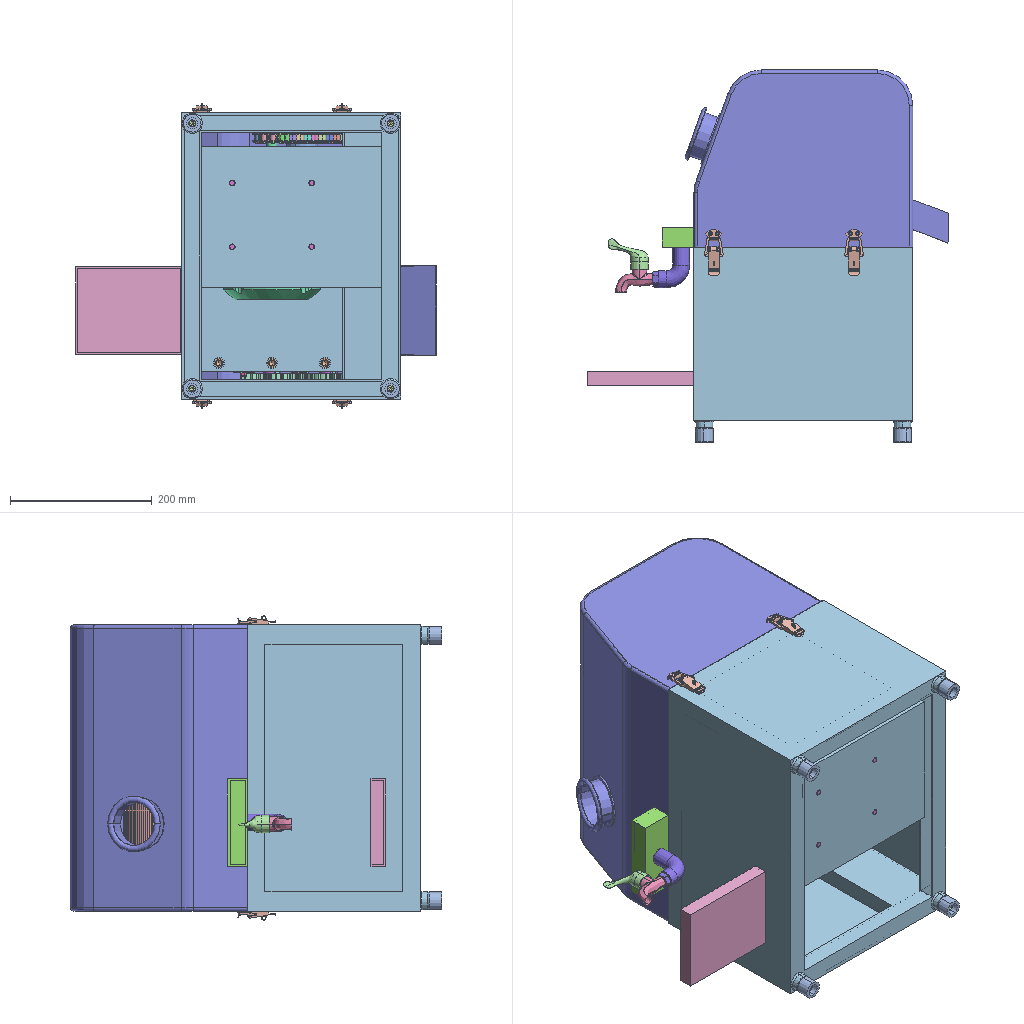Assembly | SolidWorks | 43 different items | 139 placed | box 509 x 525 x 430 mm
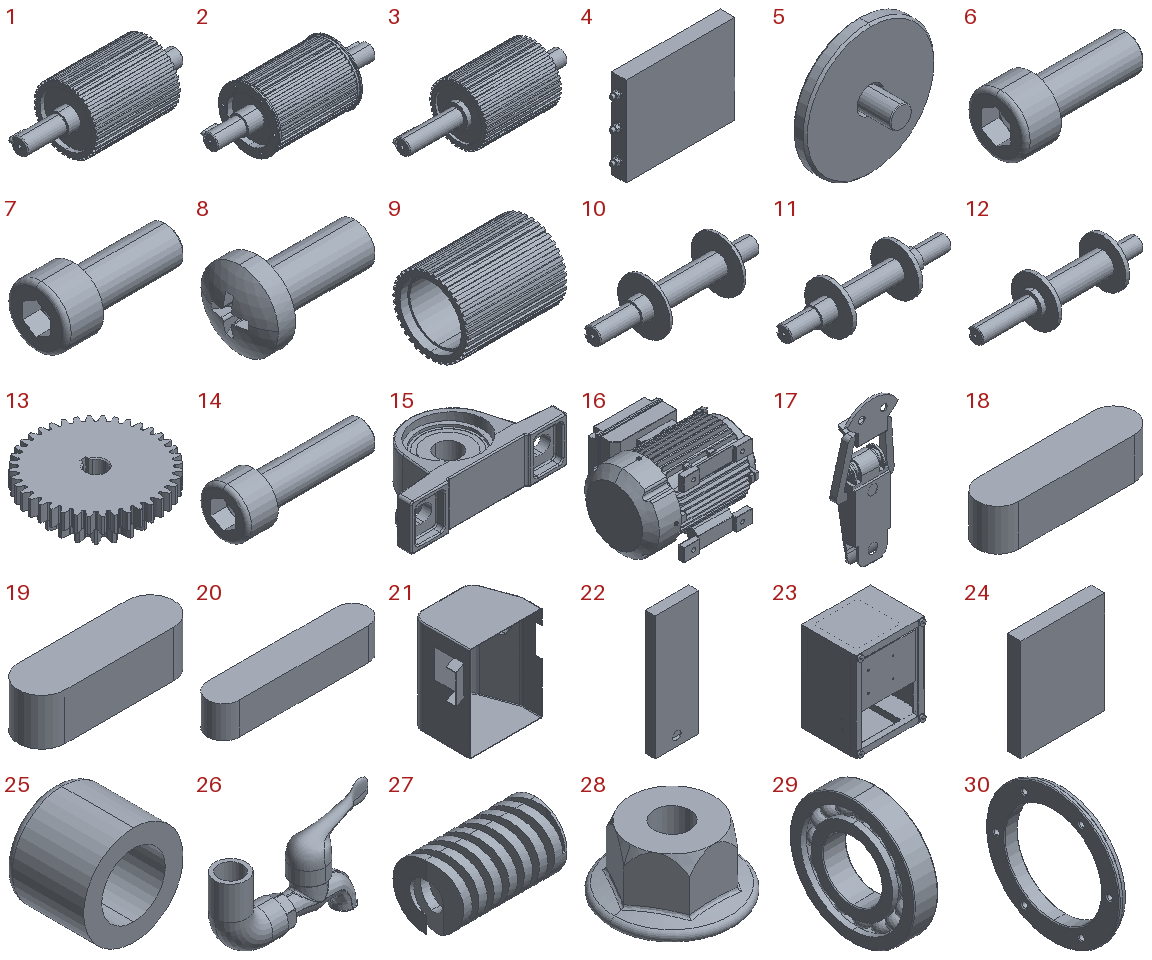Parts list (item | name | quantity | parent item | size | volume | features):
1 | (subassembly) | x1 | - | 188 x 76 x 75.929 mm | 254604 mm3 | -
2 | (subassembly) | x2 | - | 206 x 79 x 79 mm | 296188 mm3 | -
3 | (subassembly) | x1 | - | 211 x 76 x 75.929 mm | 292189 mm3 | -
4 | (subassembly) | x1 | - | 160 x 20 x 123 mm | 58465 mm3 | -
5 | (subassembly) | x10 | - | 30 x 15 x 30 mm | 2467 mm3 | -
6 | - | x4 | - | 22 x 10 x 10 mm | 844.992 mm3 | features BaseBody 1
7 | - | x4 | - | 28 x 13 x 13 mm | 1916 mm3 | features BaseBody 1
8 | - | x3 | in 4 | 15.658 x 9.5 x 9.5 mm | 430.614 mm3 | features BaseBody 1
9 | - | x4 | in 1, 2, 3 | 100 x 76 x 75.929 mm | 159717 mm3 | features BaseBody 1
10 | - | x1 | in 1 | 188 x 62 x 62 mm | 94213 mm3 | features BaseBody 1
11 | - | x2 | in 2 | 206 x 62 x 62 mm | 111425 mm3 | features BaseBody 1
12 | - | x1 | in 3 | 211 x 62 x 62 mm | 131438 mm3 | features BaseBody 1
13 | - | x1 | - | 125.77 x 125.77 x 38 mm | 253321 mm3 | features BaseBody 1
14 | - | x6 | - | 45 x 16 x 16 mm | 4425 mm3 | features BaseBody 1
15 | - | x2 | - | 127 x 73 x 37 mm | 102331 mm3 | features BaseBody 1
16 | - | x1 | - | 240 x 189 x 140.895 mm | 3047126 mm3 | features BaseBody 1
17 | - | x4 | - | 26 x 13 x 64.364 mm | 4721 mm3 | features BaseBody 1
18 | - | x1 | - | 19 x 5 x 5 mm | 448.175 mm3 | features BaseBody 1
19 | - | x7 | in 1, 2 | 20 x 6 x 6 mm | 673.646 mm3 | features BaseBody 1
20 | - | x1 | in 3 | 30 x 6 x 6 mm | 1034 mm3 | features BaseBody 1
21 | - | x1 | - | 371.669 x 250 x 404 mm | 855867 mm3 | features MoveFace 5, BaseBody 1
22 | - | x1 | - | 123 x 28 x 350 mm | 283122 mm3 | features BaseBody 1, DelFace 1, ICE 1, MoveFace 1
23 | - | x1 | - | 309 x 266.4 x 404 mm | 2740160 mm3 | features BaseBody 7, MoveFace 3, Split 2, CombineBodies 1, DelFace 1, ICE 1, MoveCopyBody 1
24 | - | x1 | in 4 | 123 x 20 x 150 mm | 56150 mm3 | features BaseBody 1
25 | - | x4 | - | 25 x 20 x 25 mm | 7114 mm3 | features BaseBody 1
26 | - | x1 | - | - | - | features BaseBody 2, RefSurface 1
27 | - | x4 | - | 35 x 20 x 20 mm | 4844 mm3 | features BaseBody 1
28 | - | x3 | in 4 | 11.8 x 11.8 x 6.2 mm | 341.044 mm3 | features BaseBody 1
29 | - | x8 | - | 8 x 42 x 42 mm | 6601 mm3 | features BaseBody 1
30 | - | x4 | in 2 | 8 x 79 x 79 mm | 11850 mm3 | features BaseBody 1, Chamfer 1, DelFace 1, MoveFace 1
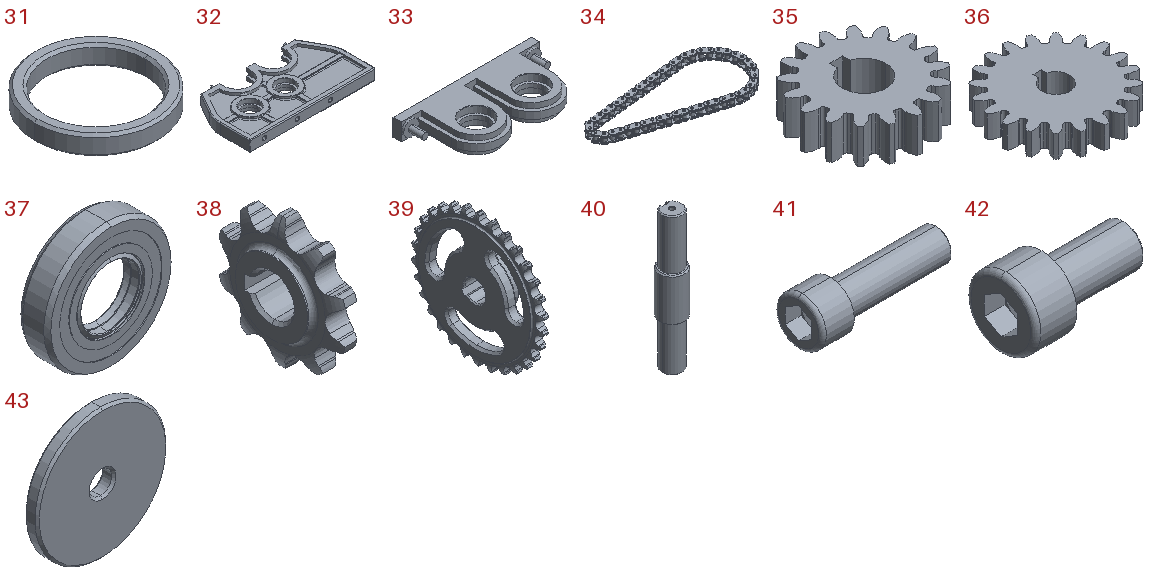31 | - | x9 | - | 25 x 25 x 4 mm | 671.515 mm3 | features BaseBody 1
32 | - | x2 | - | 285 x 151.742 x 25 mm | 571521 mm3 | features ICE 5, MoveFace 2, BaseBody 1, CombineBodies 1, DeleteBody 1, ExtruRefSurface 1, MirrorSolid 1, Split 1
33 | - | x2 | - | 200 x 95.96 x 25 mm | 244043 mm3 | features ICE 2, MoveCopyBody 2, BaseBody 1, CombineBodies 1
34 | - | x1 | - | 290.935 x 132.94 x 17.8 mm | 66914 mm3 | features BaseBody 78
35 | - | x1 | - | 56.683 x 56.908 x 16 mm | 26557 mm3 | features BaseBody 1
36 | - | x5 | - | 87.308 x 87.308 x 16 mm | 73435 mm3 | features BaseBody 1
37 | - | x7 | - | 42 x 10 x 42 mm | 3936 mm3 | features BaseBody 3
38 | - | x1 | - | 11.39 x 43.493 x 45 mm | 8237 mm3 | features BaseBody 1
39 | - | x1 | - | 20.59 x 126.465 x 127 mm | 93015 mm3 | features BaseBody 1
40 | - | x1 | - | 25 x 25 x 138.5 mm | 49958 mm3 | features BaseBody 1
41 | - | x4 | - | 52 x 18 x 18 mm | 6949 mm3 | features BaseBody 1
42 | - | x10 | in 5 | 15 x 8.5 x 8.5 mm | 438.126 mm3 | features BaseBody 1
43 | - | x10 | in 5 | 30 x 3 x 30 mm | 2029 mm3 | features BaseBody 1
Mates (type | each side: item.copy, entity, surface, feature):
Concentric | 32.1 face cylinder Cut-Extrude1 | assembly face
Concentric | assembly face | 36.1 face
Coincident | assembly face | 36.1 face
Parallel | assembly face | 36.1 face
Concentric | assembly face | 43.1 face
Coincident | assembly face | 43.1 face
Concentric | 43.1 face | 42.1 face
Coincident | 43.1 face | 42.1 face
Concentric | 33.1 face cylinder Body-Move/Copy1 | 27.1 face cylinder Input 1
Coincident | 32.2 face plane Input 1 | 27.1 face plane Input 1
Concentric | 33.2 face cylinder Body-Move/Copy1 | 27.2 face cylinder Input 1
Coincident | 32.1 face plane Input 1 | 27.2 face plane Input 1
Width | 22.1 face plane Input 1 | 22.1 face plane Input 1 | 26.1 face cylinder Input 1
Coincident | 22.1 face plane Input 1 | 26.1 face plane Input 1
Concentric | 22.1 face cylinder Cut-Extrude1 | 26.1 face cylinder Input 1
Concentric | 23.1 face cylinder Input 6 | 6.1 face cylinder Input 1
Concentric | 23.1 face cylinder Input 6 | 25.1 face cylinder Input 1
Coincident | 23.1 face plane Input 6 | 25.1 face plane Input 1
Concentric | 25.2 face cylinder Input 1 | 6.2 face cylinder Input 1
Coincident | 25.2 face plane Input 1 | 6.2 face plane Input 1
Concentric | 23.1 face cylinder Input 6 | 25.2 face cylinder Input 1
Coincident | 23.1 face plane Input 6 | 25.2 face plane Input 1
Coincident | 23.1 face plane Input 6 | 22.1 face plane Input 1
Width | 32.2 face plane Input 1 | 32.1 face plane Input 1 | 22.1 face plane Input 1 | 22.1 face plane Input 1
DistanceDim | 22.1 face plane Input 1 | 23.1 face plane Input 6
Coincident | 23.1 face plane Input 6 | 21.1 face plane Input 1
Width | 23.1 face plane Input 6 | 23.1 face plane Input 6 | 21.1 face plane Input 1 | 21.1 face plane Input 1 | 2 times
Coincident | 23.1 face plane Input 6 | 24.1 face plane Input 1
Concentric | 23.1 face cylinder Cut-Extrude1 | 8.1 face cylinder Input 1
Concentric | 23.1 face cylinder Cut-Extrude1 | 8.2 face cylinder Input 1